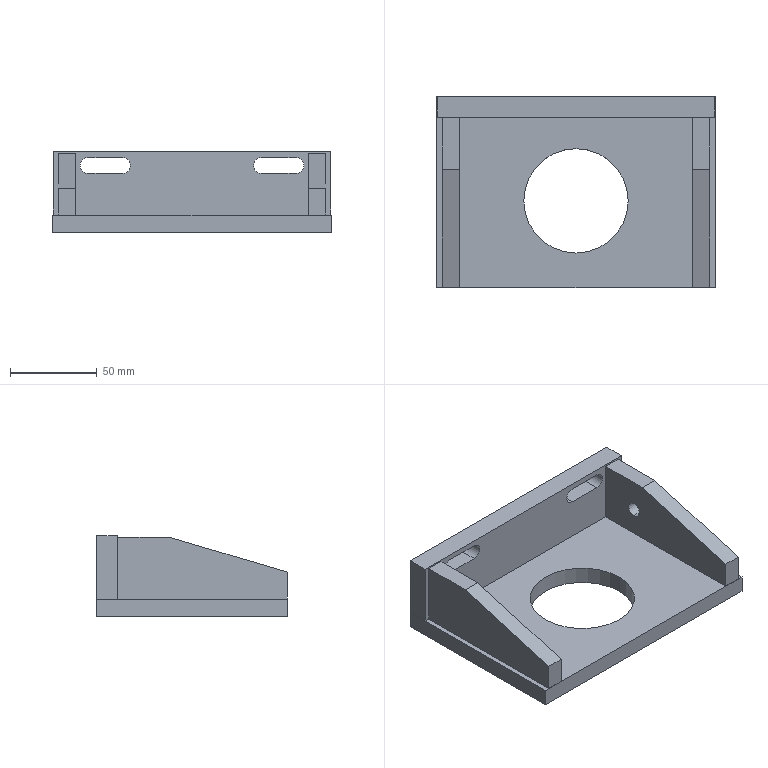Part | STEP file | 012-6-07-07 | 1 solid | 35 faces | box 160 x 110 x 46.5 mm | volume 267111 mm3 | plane 27 | cylinder 8 | commonest cylinder face diameters 9 x4 8.5 x2 60 x2